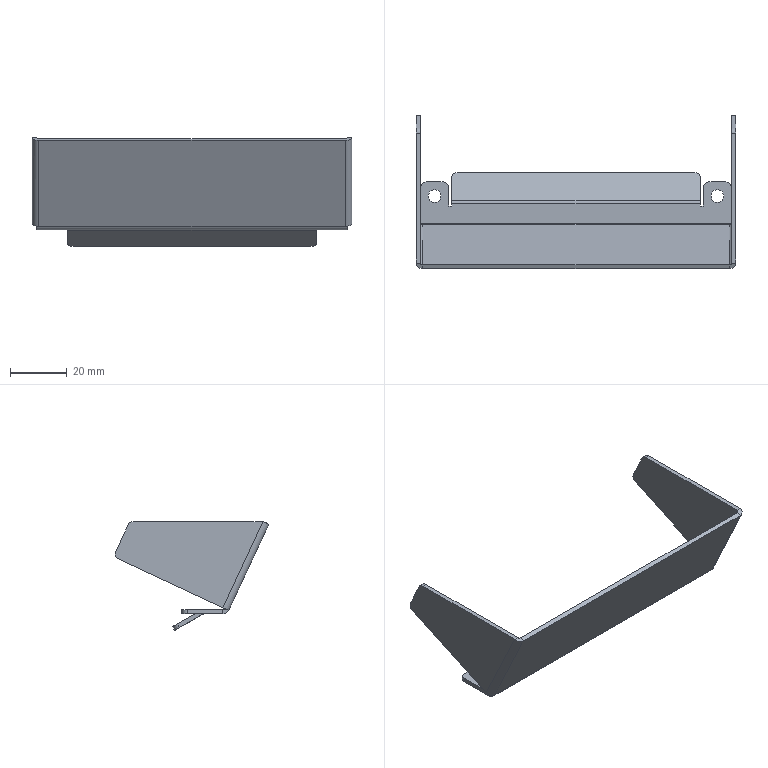Part | STEP file | 08-11 shield plate (Default) | 1 solid | 63 faces | box 113 x 54.315 x 38.465 mm | volume 11912 mm3 | plane 40 | cylinder 23 | commonest cylinder face diameters 4 x11 1.473 x4 4.473 x4 4.5 x4